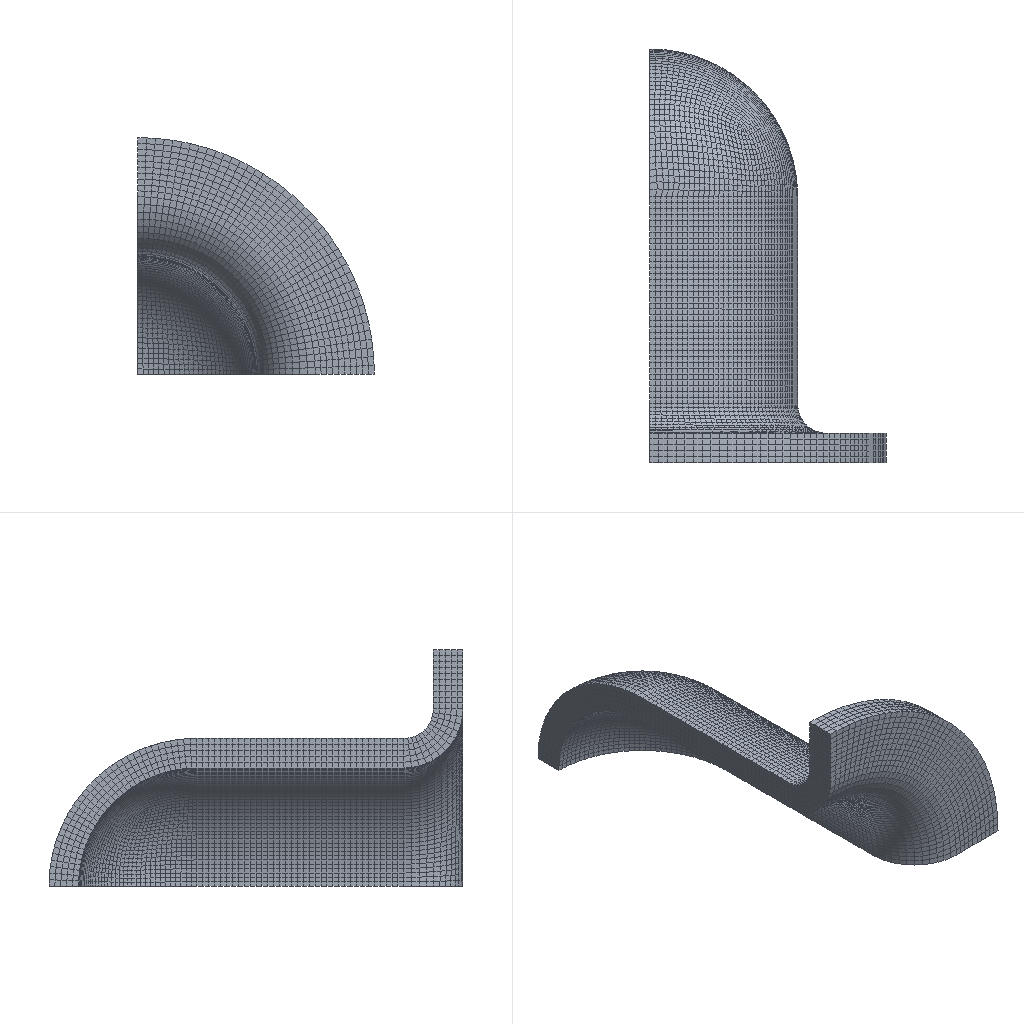Simulation study | abaqus
Set-up summary:
category,name,step,type,value,unit,region
solver,abaqus
solver,version,,,Abaqus/Standard 6.13-1
units,not stated in the deck,,not stated
analysis,deck,,static,static
load_step,Step-Static,Step-Static,static
load_step,requested,,,1
mesh,nodes,,,21222
mesh,elements,,,17115
element_type,C3D8R,,solid,17115
load,load commands in deck,,count,1
bc,support commands in deck,,count,3
material,MAT-STEEL,,in results
check,setup vs results,,match,"per instance, exact: element labels, types and connectivity; labels of the nodes the elements use; coordinates of those nodes at SINGLE_PRECISION in 1 of 1 instance(s)"
Abaqus input file, long lists of numbers shortened:
*Heading
** Job name:  Model name: Model-1
** Generated by: Abaqus/CAE 6.13-1
*Preprint, echo=NO, model=NO, history=NO, contact=NO
**
** PARTS
**
*Part, name=Part-1
*Node
      1,         600.,           0.,           0.
      2,         600.,         100.,           0.
** (21220 more lines like these left out)
*Element, type=C3D8R
   1,  152, 1545, 8471,  807,    1,   19,  735,   44
   2, 1545, 1546, 8472, 8471,   19,   20,  736,  735
** (17113 more lines like these left out)
*Nset, nset=_PickedSet2, internal, generate
     1,  21222,      1
*Elset, elset=_PickedSet2, internal, generate
     1,  17115,      1
** Section: Sect-St
*Solid Section, elset=_PickedSet2, material=Mat-Steel
,
*End Part
**
**
** ASSEMBLY
**
*Assembly, name=Assembly
**
*Instance, name=Part-1-1, part=Part-1
*End Instance
**
*Nset, nset=_PickedSet4, internal, instance=Part-1-1
    1,    4,    7,    8,   36,   37,   38,   39,   40,   41,   42,   43,   44,   62,   63,   64
   65,   66,   67,   68,   69,   70,   71,   72,   73,   74,   75,   76,   77,   78,   79,   80
** (28 more lines like these left out)
*Elset, elset=_PickedSet4, internal, instance=Part-1-1, generate
    1,  2096,     5
*Nset, nset=_PickedSet5, internal, instance=Part-1-1
    1,    2,    3,    4,    9,   10,   14,   16,   17,   18,   19,   20,   21,   22,   23,   24
   25,   26,   27,   28,   29,   30,   31,   32,   33,   34,   35,   36,   37,   38,   39,   40
** (33 more lines like these left out)
*Elset, elset=_PickedSet5, internal, instance=Part-1-1
     1,     2,     3,     4,     5,     6,     7,     8,     9,    10,    11,    12,    13,    14,    15,    16
    17,    18,    19,    20,    21,    22,    23,    24,    25,    26,    27,    28,    29,    30,    31,    32
** (27 more lines like these left out)
*Nset, nset=_PickedSet6, internal, instance=Part-1-1
    5,    6,    7,    8,   11,   12,   13,   15,   17,   18,   45,   46,   47,   48,   49,   50
   51,   52,   53,   54,   55,   56,   57,   58,   59,   60,   61,   62,   63,   64,   65,   66
** (33 more lines like these left out)
*Elset, elset=_PickedSet6, internal, instance=Part-1-1
  2051,  2052,  2053,  2054,  2055,  2056,  2057,  2058,  2059,  2060,  2061,  2062,  2063,  2064,  2065,  2066
  2067,  2068,  2069,  2070,  2071,  2072,  2073,  2074,  2075,  2076,  2077,  2078,  2079,  2080,  2081,  2082
** (27 more lines like these left out)
*Elset, elset=__PickedSurf7_S4, internal, instance=Part-1-1, generate
 2105,  4620,     5
*Elset, elset=__PickedSurf7_S2, internal, instance=Part-1-1
  4621,  4622,  4623,  4624,  4625,  4626,  4627,  4628,  4629,  4630,  4631,  4632,  4633,  4634,  4635,  4636
  4637,  4638,  4639,  4640,  4641,  4642,  4643,  4644,  4645,  4646,  4647,  4648,  4649,  4650,  4651,  4652
** (155 more lines like these left out)
*Surface, type=ELEMENT, name=_PickedSurf7, internal
__PickedSurf7_S4, S4
__PickedSurf7_S2, S2
*End Assembly
**
** MATERIALS
**
*Material, name=Mat-Steel
*Elastic
200000., 0.3
**
** BOUNDARY CONDITIONS
**
** Name: BC-1 Type: Symmetry/Antisymmetry/Encastre
*Boundary
_PickedSet4, ENCASTRE
** Name: BC-2 Type: Symmetry/Antisymmetry/Encastre
*Boundary
_PickedSet5, ZSYMM
** Name: BC-3 Type: Symmetry/Antisymmetry/Encastre
*Boundary
_PickedSet6, XSYMM
** ----------------------------------------------------------------
**
** STEP: Step-Static
**
*Step, name=Step-Static, nlgeom=NO
*Static
1., 1., 1e-05, 1.
**
** LOADS
**
** Name: Load-1   Type: Pressure
*Dsload
_PickedSurf7, P, 20.
**
** OUTPUT REQUESTS
**
*Restart, write, frequency=0
**
** FIELD OUTPUT: F-Output-1
**
*Output, field, frequency=99999
*Node Output
U,
*Element Output, directions=YES
E, S
**
** HISTORY OUTPUT: H-Output-1
**
*Output, history, variable=PRESELECT
*End Step
Results summary:
result,step,Step-Static,completed,increments=1 time=1.0/1.0
result,analysis,,,static
result,last_loadstep,,,1
result,primary field,,,U